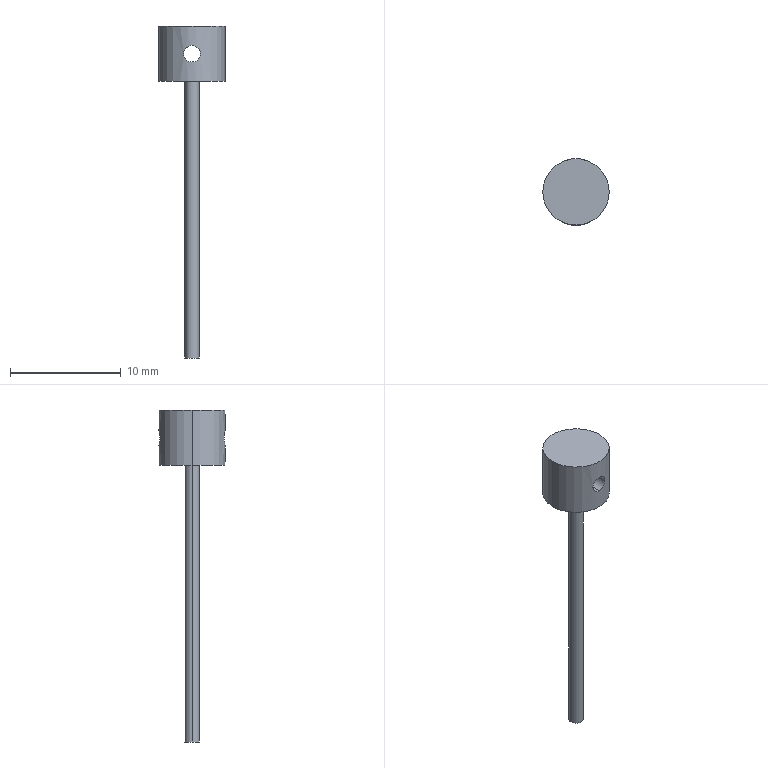Part | STEP file | detection pin | 1 solid | 9 faces | box 6 x 6 x 30 mm | volume 164.036 mm3 | cylinder 6 | plane 3 | commonest cylinder face diameters 1.3 x2 1.5 x2 6 x2
STEP:
#1=CARTESIAN_POINT('',(0.,0.,0.));
#2=DIRECTION('',(0.,0.,1.));
#3=DIRECTION('',(1.,0.,0.));
#4=AXIS2_PLACEMENT_3D('',#1,#2,#3);
#5=CARTESIAN_POINT('',(0.,3.,26.75));
#6=VERTEX_POINT('',#5);
#7=CARTESIAN_POINT('',(0.,-3.,26.75));
#8=VERTEX_POINT('',#7);
#9=CARTESIAN_POINT('',(0.,5.,26.75));
#10=DIRECTION('',(0.,-1.,0.));
#11=VECTOR('',#10,1.);
#12=LINE('',#9,#11);
#13=CARTESIAN_POINT('',(0.,5.,27.5));
#14=DIRECTION('',(0.,-1.,0.));
#15=DIRECTION('',(0.,0.,-1.));
#16=AXIS2_PLACEMENT_3D('',#13,#14,#15);
#17=CYLINDRICAL_SURFACE('',#16,0.75);
#18=CARTESIAN_POINT('',(6.283,0.));
#19=DIRECTION('',(0.,1.));
#20=VECTOR('',#19,1.);
#21=LINE('',#18,#20);
#22=(GEOMETRIC_REPRESENTATION_CONTEXT(2)PARAMETRIC_REPRESENTATION_CONTEXT()REPRESENTATION_CONTEXT('',''));
#23=DEFINITIONAL_REPRESENTATION('',(#21),#22);
#24=PCURVE('',#17,#23);
#25=CARTESIAN_POINT('',(0.,5.,27.5));
#26=DIRECTION('',(0.,-1.,0.));
#27=DIRECTION('',(0.,0.,-1.));
#28=AXIS2_PLACEMENT_3D('',#25,#26,#27);
#29=CYLINDRICAL_SURFACE('',#28,0.75);
#30=CARTESIAN_POINT('',(0.,0.));
#31=DIRECTION('',(0.,1.));
#32=VECTOR('',#31,1.);
#33=LINE('',#30,#32);
#34=(GEOMETRIC_REPRESENTATION_CONTEXT(2)PARAMETRIC_REPRESENTATION_CONTEXT()REPRESENTATION_CONTEXT('',''));
#35=DEFINITIONAL_REPRESENTATION('',(#33),#34);
#36=PCURVE('',#29,#35);
#37=SURFACE_CURVE('',#12,(#24,#36),.PCURVE_S1.);
#38=EDGE_CURVE('',#6,#8,#37,.T.);
#39=ORIENTED_EDGE('',*,*,#38,.T.);
#40=CARTESIAN_POINT('',(0.,-3.,28.25));
#41=VERTEX_POINT('',#40);
#42=CARTESIAN_POINT('',(0.,-3.,28.25));
#43=CARTESIAN_POINT('',(-0.0981,-3.,28.25));
#44=CARTESIAN_POINT('',(-0.1972,-2.995,28.23));
#45=CARTESIAN_POINT('',(-0.3778,-2.977,28.155));
#46=CARTESIAN_POINT('',(-0.4609,-2.965,28.1));
#47=CARTESIAN_POINT('',(-0.6685,-2.928,27.892));
#48=CARTESIAN_POINT('',(-0.7499,-2.905,27.698));
#49=CARTESIAN_POINT('',(-0.7501,-2.905,27.302));
#50=CARTESIAN_POINT('',(-0.6682,-2.928,27.108));
#51=CARTESIAN_POINT('',(-0.3931,-2.977,26.832));
#52=CARTESIAN_POINT('',(-0.199,-3.,26.75));
#53=CARTESIAN_POINT('',(0.,-3.,26.75));
#54=B_SPLINE_CURVE_WITH_KNOTS('',3,(#42,#43,#44,#45,#46,#47,#48,#49,#50,#51,#52,#53),.UNSPECIFIED.,.F.,.F.,(4,2,2,2,2,4),(0.002354,0.002648,0.002943,0.003531,0.004119,0.004708),.UNSPECIFIED.);
#55=CARTESIAN_POINT('',(3.142,8.));
#56=CARTESIAN_POINT('',(3.189,8.));
#57=CARTESIAN_POINT('',(3.285,7.999));
#58=CARTESIAN_POINT('',(3.428,7.993));
#59=CARTESIAN_POINT('',(3.571,7.984));
#60=CARTESIAN_POINT('',(3.713,7.973));
#61=CARTESIAN_POINT('',(3.855,7.96));
#62=CARTESIAN_POINT('',(3.998,7.946));
#63=CARTESIAN_POINT('',(4.14,7.933));
#64=CARTESIAN_POINT('',(4.283,7.922));
#65=CARTESIAN_POINT('',(4.425,7.912));
#66=CARTESIAN_POINT('',(4.568,7.906));
#67=CARTESIAN_POINT('',(4.712,7.904));
#68=CARTESIAN_POINT('',(4.856,7.906));
#69=CARTESIAN_POINT('',(4.999,7.912));
#70=CARTESIAN_POINT('',(5.142,7.922));
#71=CARTESIAN_POINT('',(5.284,7.933));
#72=CARTESIAN_POINT('',(5.426,7.946));
#73=CARTESIAN_POINT('',(5.568,7.96));
#74=CARTESIAN_POINT('',(5.71,7.972));
#75=CARTESIAN_POINT('',(5.852,7.984));
#76=CARTESIAN_POINT('',(5.995,7.993));
#77=CARTESIAN_POINT('',(6.139,7.999));
#78=CARTESIAN_POINT('',(6.235,8.));
#79=CARTESIAN_POINT('',(6.283,8.));
#80=B_SPLINE_CURVE_WITH_KNOTS('',3,(#55,#56,#57,#58,#59,#60,#61,#62,#63,#64,#65,#66,#67,#68,#69,#70,#71,#72,#73,#74,#75,#76,#77,#78,#79),.UNSPECIFIED.,.F.,.F.,(4,1,1,1,1,1,1,1,1,1,1,1,1,1,1,1,1,1,1,1,1,1,4),(0.002354,0.002461,0.002568,0.002675,0.002782,0.002889,0.002996,0.003103,0.00321,0.003317,0.003424,0.003531,0.003638,0.003745,0.003852,0.003959,0.004066,0.004173,0.00428,0.004387,0.004494,0.004601,0.004708),.QUASI_UNIFORM_KNOTS.);
#81=(GEOMETRIC_REPRESENTATION_CONTEXT(2)PARAMETRIC_REPRESENTATION_CONTEXT()REPRESENTATION_CONTEXT('',''));
#82=DEFINITIONAL_REPRESENTATION('',(#80),#81);
#83=PCURVE('',#17,#82);
#84=CARTESIAN_POINT('',(0.,0.,30.));
#85=DIRECTION('',(0.,0.,-1.));
#86=DIRECTION('',(-1.,0.,0.));
#87=AXIS2_PLACEMENT_3D('',#84,#85,#86);
#88=CYLINDRICAL_SURFACE('',#87,3.);
#89=CARTESIAN_POINT('',(4.712,1.75));
#90=CARTESIAN_POINT('',(4.724,1.75));
#91=CARTESIAN_POINT('',(4.748,1.755));
#92=CARTESIAN_POINT('',(4.783,1.778));
#93=CARTESIAN_POINT('',(4.817,1.816));
#94=CARTESIAN_POINT('',(4.848,1.867));
#95=CARTESIAN_POINT('',(4.877,1.931));
#96=CARTESIAN_POINT('',(4.903,2.007));
#97=CARTESIAN_POINT('',(4.925,2.093));
#98=CARTESIAN_POINT('',(4.942,2.187));
#99=CARTESIAN_POINT('',(4.955,2.287));
#100=CARTESIAN_POINT('',(4.963,2.392));
#101=CARTESIAN_POINT('',(4.966,2.5));
#102=CARTESIAN_POINT('',(4.963,2.608));
#103=CARTESIAN_POINT('',(4.955,2.713));
#104=CARTESIAN_POINT('',(4.942,2.813));
#105=CARTESIAN_POINT('',(4.925,2.907));
#106=CARTESIAN_POINT('',(4.903,2.993));
#107=CARTESIAN_POINT('',(4.878,3.068));
#108=CARTESIAN_POINT('',(4.849,3.132));
#109=CARTESIAN_POINT('',(4.817,3.183));
#110=CARTESIAN_POINT('',(4.784,3.221));
#111=CARTESIAN_POINT('',(4.748,3.245));
#112=CARTESIAN_POINT('',(4.724,3.25));
#113=CARTESIAN_POINT('',(4.712,3.25));
#114=B_SPLINE_CURVE_WITH_KNOTS('',3,(#89,#90,#91,#92,#93,#94,#95,#96,#97,#98,#99,#100,#101,#102,#103,#104,#105,#106,#107,#108,#109,#110,#111,#112,#113),.UNSPECIFIED.,.F.,.F.,(4,1,1,1,1,1,1,1,1,1,1,1,1,1,1,1,1,1,1,1,1,1,4),(0.002354,0.002461,0.002568,0.002675,0.002782,0.002889,0.002996,0.003103,0.00321,0.003317,0.003424,0.003531,0.003638,0.003745,0.003852,0.003959,0.004066,0.004173,0.00428,0.004387,0.004494,0.004601,0.004708),.QUASI_UNIFORM_KNOTS.);
#115=(GEOMETRIC_REPRESENTATION_CONTEXT(2)PARAMETRIC_REPRESENTATION_CONTEXT()REPRESENTATION_CONTEXT('',''));
#116=DEFINITIONAL_REPRESENTATION('',(#114),#115);
#117=PCURVE('',#88,#116);
#118=SURFACE_CURVE('',#54,(#83,#117),.PCURVE_S1.);
#119=EDGE_CURVE('',#41,#8,#118,.T.);
#120=ORIENTED_EDGE('',*,*,#119,.F.);
#121=CARTESIAN_POINT('',(0.,3.,28.25));
#122=VERTEX_POINT('',#121);
#123=CARTESIAN_POINT('',(0.,5.,28.25));
#124=DIRECTION('',(0.,-1.,0.));
#125=VECTOR('',#124,1.);
#126=LINE('',#123,#125);
#127=CARTESIAN_POINT('',(3.142,0.));
#128=DIRECTION('',(0.,1.));
#129=VECTOR('',#128,1.);
#130=LINE('',#127,#129);
#131=(GEOMETRIC_REPRESENTATION_CONTEXT(2)PARAMETRIC_REPRESENTATION_CONTEXT()REPRESENTATION_CONTEXT('',''));
#132=DEFINITIONAL_REPRESENTATION('',(#130),#131);
#133=PCURVE('',#17,#132);
#134=CARTESIAN_POINT('',(3.142,0.));
#135=DIRECTION('',(0.,1.));
#136=VECTOR('',#135,1.);
#137=LINE('',#134,#136);
#138=(GEOMETRIC_REPRESENTATION_CONTEXT(2)PARAMETRIC_REPRESENTATION_CONTEXT()REPRESENTATION_CONTEXT('',''));
#139=DEFINITIONAL_REPRESENTATION('',(#137),#138);
#140=PCURVE('',#29,#139);
#141=SURFACE_CURVE('',#126,(#133,#140),.PCURVE_S1.);
#142=EDGE_CURVE('',#122,#41,#141,.T.);
#143=ORIENTED_EDGE('',*,*,#142,.F.);
#144=CARTESIAN_POINT('',(0.,3.,26.75));
#145=CARTESIAN_POINT('',(-0.09953,3.,26.75));
#146=CARTESIAN_POINT('',(-0.1972,2.995,26.77));
#147=CARTESIAN_POINT('',(-0.3787,2.977,26.845));
#148=CARTESIAN_POINT('',(-0.4616,2.965,26.901));
#149=CARTESIAN_POINT('',(-0.5994,2.94,27.039));
#150=CARTESIAN_POINT('',(-0.6552,2.928,27.122));
#151=CARTESIAN_POINT('',(-0.7301,2.91,27.302));
#152=CARTESIAN_POINT('',(-0.75,2.905,27.401));
#153=CARTESIAN_POINT('',(-0.75,2.905,27.598));
#154=CARTESIAN_POINT('',(-0.7305,2.91,27.696));
#155=CARTESIAN_POINT('',(-0.6549,2.928,27.879));
#156=CARTESIAN_POINT('',(-0.5997,2.94,27.961));
#157=CARTESIAN_POINT('',(-0.4607,2.965,28.1));
#158=CARTESIAN_POINT('',(-0.3781,2.977,28.155));
#159=CARTESIAN_POINT('',(-0.197,2.995,28.23));
#160=CARTESIAN_POINT('',(-0.09813,3.,28.25));
#161=CARTESIAN_POINT('',(0.,3.,28.25));
#162=B_SPLINE_CURVE_WITH_KNOTS('',3,(#144,#145,#146,#147,#148,#149,#150,#151,#152,#153,#154,#155,#156,#157,#158,#159,#160,#161),.UNSPECIFIED.,.F.,.F.,(4,2,2,2,2,2,2,2,4),(0.,0.0002943,0.0005886,0.0008828,0.001177,0.001471,0.001766,0.00206,0.002354),.UNSPECIFIED.);
#163=CARTESIAN_POINT('',(6.283,2.));
#164=CARTESIAN_POINT('',(6.259,2.));
#165=CARTESIAN_POINT('',(6.211,2.));
#166=CARTESIAN_POINT('',(6.139,2.002));
#167=CARTESIAN_POINT('',(6.068,2.004));
#168=CARTESIAN_POINT('',(5.996,2.007));
#169=CARTESIAN_POINT('',(5.925,2.011));
#170=CARTESIAN_POINT('',(5.853,2.016));
#171=CARTESIAN_POINT('',(5.782,2.022));
#172=CARTESIAN_POINT('',(5.711,2.028));
#173=CARTESIAN_POINT('',(5.639,2.034));
#174=CARTESIAN_POINT('',(5.568,2.041));
#175=CARTESIAN_POINT('',(5.497,2.047));
#176=CARTESIAN_POINT('',(5.427,2.054));
#177=CARTESIAN_POINT('',(5.355,2.061));
#178=CARTESIAN_POINT('',(5.284,2.067));
#179=CARTESIAN_POINT('',(5.213,2.073));
#180=CARTESIAN_POINT('',(5.142,2.079));
#181=CARTESIAN_POINT('',(5.071,2.084));
#182=CARTESIAN_POINT('',(4.999,2.088));
#183=CARTESIAN_POINT('',(4.928,2.091));
#184=CARTESIAN_POINT('',(4.856,2.093));
#185=CARTESIAN_POINT('',(4.784,2.095));
#186=CARTESIAN_POINT('',(4.713,2.095));
#187=CARTESIAN_POINT('',(4.641,2.095));
#188=CARTESIAN_POINT('',(4.57,2.093));
#189=CARTESIAN_POINT('',(4.498,2.091));
#190=CARTESIAN_POINT('',(4.427,2.088));
#191=CARTESIAN_POINT('',(4.355,2.084));
#192=CARTESIAN_POINT('',(4.283,2.079));
#193=CARTESIAN_POINT('',(4.212,2.073));
#194=CARTESIAN_POINT('',(4.141,2.067));
#195=CARTESIAN_POINT('',(4.069,2.061));
#196=CARTESIAN_POINT('',(3.998,2.054));
#197=CARTESIAN_POINT('',(3.927,2.047));
#198=CARTESIAN_POINT('',(3.855,2.04));
#199=CARTESIAN_POINT('',(3.784,2.034));
#200=CARTESIAN_POINT('',(3.713,2.027));
#201=CARTESIAN_POINT('',(3.642,2.022));
#202=CARTESIAN_POINT('',(3.571,2.016));
#203=CARTESIAN_POINT('',(3.499,2.011));
#204=CARTESIAN_POINT('',(3.428,2.007));
#205=CARTESIAN_POINT('',(3.356,2.004));
#206=CARTESIAN_POINT('',(3.285,2.002));
#207=CARTESIAN_POINT('',(3.213,2.));
#208=CARTESIAN_POINT('',(3.165,2.));
#209=CARTESIAN_POINT('',(3.142,2.));
#210=B_SPLINE_CURVE_WITH_KNOTS('',3,(#163,#164,#165,#166,#167,#168,#169,#170,#171,#172,#173,#174,#175,#176,#177,#178,#179,#180,#181,#182,#183,#184,#185,#186,#187,#188,#189,#190,#191,#192,#193,#194,#195,#196,#197,#198,#199,#200,#201,#202,#203,#204,#205,#206,#207,#208,#209),.UNSPECIFIED.,.F.,.F.,(4,1,1,1,1,1,1,1,1,1,1,1,1,1,1,1,1,1,1,1,1,1,1,1,1,1,1,1,1,1,1,1,1,1,1,1,1,1,1,1,1,1,1,1,4),(0.,0.0000535,0.000107,0.0001605,0.000214,0.0002675,0.000321,0.0003745,0.000428,0.0004815,0.000535,0.0005886,0.0006421,0.0006956,0.0007491,0.0008026,0.0008561,0.0009096,0.0009631,0.001017,0.00107,0.001124,0.001177,0.001231,0.001284,0.001338,0.001391,0.001445,0.001498,0.001552,0.001605,0.001659,0.001712,0.001766,0.001819,0.001873,0.001926,0.00198,0.002033,0.002087,0.00214,0.002194,0.002247,0.002301,0.002354),.QUASI_UNIFORM_KNOTS.);
#211=(GEOMETRIC_REPRESENTATION_CONTEXT(2)PARAMETRIC_REPRESENTATION_CONTEXT()REPRESENTATION_CONTEXT('',''));
#212=DEFINITIONAL_REPRESENTATION('',(#210),#211);
#213=PCURVE('',#17,#212);
#214=CARTESIAN_POINT('',(0.,0.,30.));
#215=DIRECTION('',(0.,0.,-1.));
#216=DIRECTION('',(-1.,0.,0.));
#217=AXIS2_PLACEMENT_3D('',#214,#215,#216);
#218=CYLINDRICAL_SURFACE('',#217,3.);
#219=CARTESIAN_POINT('',(1.571,3.25));
#220=CARTESIAN_POINT('',(1.565,3.25));
#221=CARTESIAN_POINT('',(1.553,3.249));
#222=CARTESIAN_POINT('',(1.535,3.243));
#223=CARTESIAN_POINT('',(1.517,3.233));
#224=CARTESIAN_POINT('',(1.5,3.22));
#225=CARTESIAN_POINT('',(1.483,3.203));
#226=CARTESIAN_POINT('',(1.466,3.182));
#227=CARTESIAN_POINT('',(1.45,3.158));
#228=CARTESIAN_POINT('',(1.435,3.131));
#229=CARTESIAN_POINT('',(1.42,3.1));
#230=CARTESIAN_POINT('',(1.406,3.067));
#231=CARTESIAN_POINT('',(1.393,3.031));
#232=CARTESIAN_POINT('',(1.381,2.992));
#233=CARTESIAN_POINT('',(1.369,2.95));
#234=CARTESIAN_POINT('',(1.359,2.906));
#235=CARTESIAN_POINT('',(1.349,2.86));
#236=CARTESIAN_POINT('',(1.341,2.812));
#237=CARTESIAN_POINT('',(1.334,2.763));
#238=CARTESIAN_POINT('',(1.328,2.712));
#239=CARTESIAN_POINT('',(1.324,2.66));
#240=CARTESIAN_POINT('',(1.321,2.607));
#241=CARTESIAN_POINT('',(1.319,2.554));
#242=CARTESIAN_POINT('',(1.318,2.5));
#243=CARTESIAN_POINT('',(1.319,2.447));
#244=CARTESIAN_POINT('',(1.321,2.393));
#245=CARTESIAN_POINT('',(1.324,2.34));
#246=CARTESIAN_POINT('',(1.328,2.288));
#247=CARTESIAN_POINT('',(1.334,2.237));
#248=CARTESIAN_POINT('',(1.341,2.188));
#249=CARTESIAN_POINT('',(1.349,2.14));
#250=CARTESIAN_POINT('',(1.359,2.094));
#251=CARTESIAN_POINT('',(1.369,2.05));
#252=CARTESIAN_POINT('',(1.381,2.008));
#253=CARTESIAN_POINT('',(1.393,1.969));
#254=CARTESIAN_POINT('',(1.406,1.933));
#255=CARTESIAN_POINT('',(1.42,1.899));
#256=CARTESIAN_POINT('',(1.435,1.869));
#257=CARTESIAN_POINT('',(1.451,1.841));
#258=CARTESIAN_POINT('',(1.467,1.817));
#259=CARTESIAN_POINT('',(1.483,1.797));
#260=CARTESIAN_POINT('',(1.5,1.78));
#261=CARTESIAN_POINT('',(1.517,1.767));
#262=CARTESIAN_POINT('',(1.535,1.757));
#263=CARTESIAN_POINT('',(1.553,1.751));
#264=CARTESIAN_POINT('',(1.565,1.75));
#265=CARTESIAN_POINT('',(1.571,1.75));
#266=B_SPLINE_CURVE_WITH_KNOTS('',3,(#219,#220,#221,#222,#223,#224,#225,#226,#227,#228,#229,#230,#231,#232,#233,#234,#235,#236,#237,#238,#239,#240,#241,#242,#243,#244,#245,#246,#247,#248,#249,#250,#251,#252,#253,#254,#255,#256,#257,#258,#259,#260,#261,#262,#263,#264,#265),.UNSPECIFIED.,.F.,.F.,(4,1,1,1,1,1,1,1,1,1,1,1,1,1,1,1,1,1,1,1,1,1,1,1,1,1,1,1,1,1,1,1,1,1,1,1,1,1,1,1,1,1,1,1,4),(0.,0.0000535,0.000107,0.0001605,0.000214,0.0002675,0.000321,0.0003745,0.000428,0.0004815,0.000535,0.0005886,0.0006421,0.0006956,0.0007491,0.0008026,0.0008561,0.0009096,0.0009631,0.001017,0.00107,0.001124,0.001177,0.001231,0.001284,0.001338,0.001391,0.001445,0.001498,0.001552,0.001605,0.001659,0.001712,0.001766,0.001819,0.001873,0.001926,0.00198,0.002033,0.002087,0.00214,0.002194,0.002247,0.002301,0.002354),.QUASI_UNIFORM_KNOTS.);
#267=(GEOMETRIC_REPRESENTATION_CONTEXT(2)PARAMETRIC_REPRESENTATION_CONTEXT()REPRESENTATION_CONTEXT('',''));
#268=DEFINITIONAL_REPRESENTATION('',(#266),#267);
#269=PCURVE('',#218,#268);
#270=SURFACE_CURVE('',#162,(#213,#269),.PCURVE_S1.);
#271=EDGE_CURVE('',#6,#122,#270,.T.);
#272=ORIENTED_EDGE('',*,*,#271,.F.);
#273=EDGE_LOOP('',(#39,#120,#143,#272));
#274=FACE_BOUND('',#273,.F.);
#275=ADVANCED_FACE('',(#274),#17,.F.);
#276=CARTESIAN_POINT('',(0.65,0.,25.));
#277=VERTEX_POINT('',#276);
#278=CARTESIAN_POINT('',(-0.65,0.,25.));
#279=VERTEX_POINT('',#278);
#280=CARTESIAN_POINT('',(0.,0.,25.));
#281=DIRECTION('',(0.,0.,1.));
#282=DIRECTION('',(1.,0.,0.));
#283=AXIS2_PLACEMENT_3D('',#280,#281,#282);
#284=CIRCLE('',#283,0.65);
#285=CARTESIAN_POINT('',(0.,0.,25.));
#286=DIRECTION('',(0.,0.,-1.));
#287=DIRECTION('',(-1.,0.,0.));
#288=AXIS2_PLACEMENT_3D('',#285,#286,#287);
#289=CYLINDRICAL_SURFACE('',#288,0.65);
#290=CARTESIAN_POINT('',(3.142,0.));
#291=DIRECTION('',(-1.,0.));
#292=VECTOR('',#291,1.);
#293=LINE('',#290,#292);
#294=(GEOMETRIC_REPRESENTATION_CONTEXT(2)PARAMETRIC_REPRESENTATION_CONTEXT()REPRESENTATION_CONTEXT('',''));
#295=DEFINITIONAL_REPRESENTATION('',(#293),#294);
#296=PCURVE('',#289,#295);
#297=CARTESIAN_POINT('',(0.,0.,25.));
#298=DIRECTION('',(0.,0.,1.));
#299=DIRECTION('',(1.,0.,0.));
#300=AXIS2_PLACEMENT_3D('',#297,#298,#299);
#301=PLANE('',#300);
#302=CARTESIAN_POINT('',(0.,0.));
#303=DIRECTION('',(1.,0.));
#304=AXIS2_PLACEMENT_2D('',#302,#303);
#305=CIRCLE('',#304,0.65);
#306=(GEOMETRIC_REPRESENTATION_CONTEXT(2)PARAMETRIC_REPRESENTATION_CONTEXT()REPRESENTATION_CONTEXT('',''));
#307=DEFINITIONAL_REPRESENTATION('',(#305),#306);
#308=PCURVE('',#301,#307);
#309=SURFACE_CURVE('',#284,(#296,#308),.PCURVE_S1.);
#310=EDGE_CURVE('',#277,#279,#309,.T.);
#311=ORIENTED_EDGE('',*,*,#310,.F.);
#312=CARTESIAN_POINT('',(0.65,0.,0.));
#313=VERTEX_POINT('',#312);
#314=CARTESIAN_POINT('',(0.65,0.,25.));
#315=DIRECTION('',(0.,0.,-1.));
#316=VECTOR('',#315,1.);
#317=LINE('',#314,#316);
#318=CARTESIAN_POINT('',(3.142,0.));
#319=DIRECTION('',(0.,1.));
#320=VECTOR('',#319,1.);
#321=LINE('',#318,#320);
#322=(GEOMETRIC_REPRESENTATION_CONTEXT(2)PARAMETRIC_REPRESENTATION_CONTEXT()REPRESENTATION_CONTEXT('',''));
#323=DEFINITIONAL_REPRESENTATION('',(#321),#322);
#324=PCURVE('',#289,#323);
#325=CARTESIAN_POINT('',(0.,0.,25.));
#326=DIRECTION('',(0.,0.,-1.));
#327=DIRECTION('',(-1.,0.,0.));
#328=AXIS2_PLACEMENT_3D('',#325,#326,#327);
#329=CYLINDRICAL_SURFACE('',#328,0.65);
#330=CARTESIAN_POINT('',(3.142,0.));
#331=DIRECTION('',(0.,1.));
#332=VECTOR('',#331,1.);
#333=LINE('',#330,#332);
#334=(GEOMETRIC_REPRESENTATION_CONTEXT(2)PARAMETRIC_REPRESENTATION_CONTEXT()REPRESENTATION_CONTEXT('',''));
#335=DEFINITIONAL_REPRESENTATION('',(#333),#334);
#336=PCURVE('',#329,#335);
#337=SURFACE_CURVE('',#317,(#324,#336),.PCURVE_S1.);
#338=EDGE_CURVE('',#277,#313,#337,.T.);
#339=ORIENTED_EDGE('',*,*,#338,.T.);
#340=CARTESIAN_POINT('',(-0.65,0.,0.));
#341=VERTEX_POINT('',#340);
#342=CARTESIAN_POINT('',(0.,0.,0.));
#343=DIRECTION('',(0.,0.,1.));
#344=DIRECTION('',(1.,0.,0.));
#345=AXIS2_PLACEMENT_3D('',#342,#343,#344);
#346=CIRCLE('',#345,0.65);
#347=CARTESIAN_POINT('',(3.142,25.));
#348=DIRECTION('',(-1.,0.));
#349=VECTOR('',#348,1.);
#350=LINE('',#347,#349);
#351=(GEOMETRIC_REPRESENTATION_CONTEXT(2)PARAMETRIC_REPRESENTATION_CONTEXT()REPRESENTATION_CONTEXT('',''));
#352=DEFINITIONAL_REPRESENTATION('',(#350),#351);
#353=PCURVE('',#289,#352);
#354=CARTESIAN_POINT('',(0.,0.,0.));
#355=DIRECTION('',(0.,0.,1.));
#356=DIRECTION('',(1.,0.,0.));
#357=AXIS2_PLACEMENT_3D('',#354,#355,#356);
#358=PLANE('',#357);
#359=CARTESIAN_POINT('',(0.,0.));
#360=DIRECTION('',(1.,0.));
#361=AXIS2_PLACEMENT_2D('',#359,#360);
#362=CIRCLE('',#361,0.65);
#363=(GEOMETRIC_REPRESENTATION_CONTEXT(2)PARAMETRIC_REPRESENTATION_CONTEXT()REPRESENTATION_CONTEXT('',''));
#364=DEFINITIONAL_REPRESENTATION('',(#362),#363);
#365=PCURVE('',#358,#364);
#366=SURFACE_CURVE('',#346,(#353,#365),.PCURVE_S1.);
#367=EDGE_CURVE('',#313,#341,#366,.T.);
#368=ORIENTED_EDGE('',*,*,#367,.T.);
#369=CARTESIAN_POINT('',(-0.65,0.,25.));
#370=DIRECTION('',(0.,0.,-1.));
#371=VECTOR('',#370,1.);
#372=LINE('',#369,#371);
#373=CARTESIAN_POINT('',(0.,0.));
#374=DIRECTION('',(0.,1.));
#375=VECTOR('',#374,1.);
#376=LINE('',#373,#375);
#377=(GEOMETRIC_REPRESENTATION_CONTEXT(2)PARAMETRIC_REPRESENTATION_CONTEXT()REPRESENTATION_CONTEXT('',''));
#378=DEFINITIONAL_REPRESENTATION('',(#376),#377);
#379=PCURVE('',#289,#378);
#380=CARTESIAN_POINT('',(6.283,0.));
#381=DIRECTION('',(0.,1.));
#382=VECTOR('',#381,1.);
#383=LINE('',#380,#382);
#384=(GEOMETRIC_REPRESENTATION_CONTEXT(2)PARAMETRIC_REPRESENTATION_CONTEXT()REPRESENTATION_CONTEXT('',''));
#385=DEFINITIONAL_REPRESENTATION('',(#383),#384);
#386=PCURVE('',#329,#385);
#387=SURFACE_CURVE('',#372,(#379,#386),.PCURVE_S1.);
#388=EDGE_CURVE('',#279,#341,#387,.T.);
#389=ORIENTED_EDGE('',*,*,#388,.F.);
#390=EDGE_LOOP('',(#311,#339,#368,#389));
#391=FACE_BOUND('',#390,.T.);
#392=ADVANCED_FACE('',(#391),#289,.T.);
#393=ORIENTED_EDGE('',*,*,#271,.F.);
#394=CARTESIAN_POINT('',(0.,3.,28.25));
#395=CARTESIAN_POINT('',(0.0981,3.,28.25));
#396=CARTESIAN_POINT('',(0.1972,2.995,28.23));
#397=CARTESIAN_POINT('',(0.3778,2.977,28.155));
#398=CARTESIAN_POINT('',(0.4609,2.965,28.1));
#399=CARTESIAN_POINT('',(0.6685,2.928,27.892));
#400=CARTESIAN_POINT('',(0.7499,2.905,27.698));
#401=CARTESIAN_POINT('',(0.7501,2.905,27.302));
#402=CARTESIAN_POINT('',(0.6682,2.928,27.108));
#403=CARTESIAN_POINT('',(0.3931,2.977,26.832));
#404=CARTESIAN_POINT('',(0.199,3.,26.75));
#405=CARTESIAN_POINT('',(0.,3.,26.75));
#406=B_SPLINE_CURVE_WITH_KNOTS('',3,(#394,#395,#396,#397,#398,#399,#400,#401,#402,#403,#404,#405),.UNSPECIFIED.,.F.,.F.,(4,2,2,2,2,4),(0.002354,0.002648,0.002943,0.003531,0.004119,0.004708),.UNSPECIFIED.);
#407=CARTESIAN_POINT('',(1.571,1.75));
#408=CARTESIAN_POINT('',(1.583,1.75));
#409=CARTESIAN_POINT('',(1.607,1.755));
#410=CARTESIAN_POINT('',(1.642,1.778));
#411=CARTESIAN_POINT('',(1.675,1.816));
#412=CARTESIAN_POINT('',(1.707,1.867));
#413=CARTESIAN_POINT('',(1.736,1.931));
#414=CARTESIAN_POINT('',(1.761,2.007));
#415=CARTESIAN_POINT('',(1.783,2.093));
#416=CARTESIAN_POINT('',(1.801,2.187));
#417=CARTESIAN_POINT('',(1.814,2.287));
#418=CARTESIAN_POINT('',(1.822,2.392));
#419=CARTESIAN_POINT('',(1.824,2.5));
#420=CARTESIAN_POINT('',(1.822,2.608));
#421=CARTESIAN_POINT('',(1.814,2.713));
#422=CARTESIAN_POINT('',(1.801,2.813));
#423=CARTESIAN_POINT('',(1.783,2.907));
#424=CARTESIAN_POINT('',(1.761,2.993));
#425=CARTESIAN_POINT('',(1.736,3.068));
#426=CARTESIAN_POINT('',(1.707,3.132));
#427=CARTESIAN_POINT('',(1.676,3.183));
#428=CARTESIAN_POINT('',(1.642,3.221));
#429=CARTESIAN_POINT('',(1.607,3.245));
#430=CARTESIAN_POINT('',(1.583,3.25));
#431=CARTESIAN_POINT('',(1.571,3.25));
#432=B_SPLINE_CURVE_WITH_KNOTS('',3,(#407,#408,#409,#410,#411,#412,#413,#414,#415,#416,#417,#418,#419,#420,#421,#422,#423,#424,#425,#426,#427,#428,#429,#430,#431),.UNSPECIFIED.,.F.,.F.,(4,1,1,1,1,1,1,1,1,1,1,1,1,1,1,1,1,1,1,1,1,1,4),(0.002354,0.002461,0.002568,0.002675,0.002782,0.002889,0.002996,0.003103,0.00321,0.003317,0.003424,0.003531,0.003638,0.003745,0.003852,0.003959,0.004066,0.004173,0.00428,0.004387,0.004494,0.004601,0.004708),.QUASI_UNIFORM_KNOTS.);
#433=(GEOMETRIC_REPRESENTATION_CONTEXT(2)PARAMETRIC_REPRESENTATION_CONTEXT()REPRESENTATION_CONTEXT('',''));
#434=DEFINITIONAL_REPRESENTATION('',(#432),#433);
#435=PCURVE('',#218,#434);
#436=CARTESIAN_POINT('',(3.142,2.));
#437=CARTESIAN_POINT('',(3.094,2.));
#438=CARTESIAN_POINT('',(2.999,2.001));
#439=CARTESIAN_POINT('',(2.855,2.007));
#440=CARTESIAN_POINT('',(2.713,2.016));
#441=CARTESIAN_POINT('',(2.57,2.027));
#442=CARTESIAN_POINT('',(2.428,2.04));
#443=CARTESIAN_POINT('',(2.285,2.054));
#444=CARTESIAN_POINT('',(2.143,2.067));
#445=CARTESIAN_POINT('',(2.001,2.078));
#446=CARTESIAN_POINT('',(1.858,2.088));
#447=CARTESIAN_POINT('',(1.715,2.094));
#448=CARTESIAN_POINT('',(1.571,2.096));
#449=CARTESIAN_POINT('',(1.427,2.094));
#450=CARTESIAN_POINT('',(1.284,2.088));
#451=CARTESIAN_POINT('',(1.141,2.078));
#452=CARTESIAN_POINT('',(0.9987,2.067));
#453=CARTESIAN_POINT('',(0.8567,2.054));
#454=CARTESIAN_POINT('',(0.7152,2.04));
#455=CARTESIAN_POINT('',(0.5733,2.028));
#456=CARTESIAN_POINT('',(0.4308,2.016));
#457=CARTESIAN_POINT('',(0.2878,2.007));
#458=CARTESIAN_POINT('',(0.1443,2.001));
#459=CARTESIAN_POINT('',(0.04821,2.));
#460=CARTESIAN_POINT('',(0.,2.));
#461=B_SPLINE_CURVE_WITH_KNOTS('',3,(#436,#437,#438,#439,#440,#441,#442,#443,#444,#445,#446,#447,#448,#449,#450,#451,#452,#453,#454,#455,#456,#457,#458,#459,#460),.UNSPECIFIED.,.F.,.F.,(4,1,1,1,1,1,1,1,1,1,1,1,1,1,1,1,1,1,1,1,1,1,4),(0.002354,0.002461,0.002568,0.002675,0.002782,0.002889,0.002996,0.003103,0.00321,0.003317,0.003424,0.003531,0.003638,0.003745,0.003852,0.003959,0.004066,0.004173,0.00428,0.004387,0.004494,0.004601,0.004708),.QUASI_UNIFORM_KNOTS.);
#462=(GEOMETRIC_REPRESENTATION_CONTEXT(2)PARAMETRIC_REPRESENTATION_CONTEXT()REPRESENTATION_CONTEXT('',''));
#463=DEFINITIONAL_REPRESENTATION('',(#461),#462);
#464=PCURVE('',#29,#463);
#465=SURFACE_CURVE('',#406,(#435,#464),.PCURVE_S1.);
#466=EDGE_CURVE('',#122,#6,#465,.T.);
#467=ORIENTED_EDGE('',*,*,#466,.F.);
#468=EDGE_LOOP('',(#393,#467));
#469=FACE_BOUND('',#468,.T.);
#470=CARTESIAN_POINT('',(3.,0.,30.));
#471=VERTEX_POINT('',#470);
#472=CARTESIAN_POINT('',(-3.,0.,30.));
#473=VERTEX_POINT('',#472);
#474=CARTESIAN_POINT('',(0.,0.,30.));
#475=DIRECTION('',(0.,0.,1.));
#476=DIRECTION('',(1.,0.,0.));
#477=AXIS2_PLACEMENT_3D('',#474,#475,#476);
#478=CIRCLE('',#477,3.);
#479=CARTESIAN_POINT('',(3.142,0.));
#480=DIRECTION('',(-1.,0.));
#481=VECTOR('',#480,1.);
#482=LINE('',#479,#481);
#483=(GEOMETRIC_REPRESENTATION_CONTEXT(2)PARAMETRIC_REPRESENTATION_CONTEXT()REPRESENTATION_CONTEXT('',''));
#484=DEFINITIONAL_REPRESENTATION('',(#482),#483);
#485=PCURVE('',#218,#484);
#486=CARTESIAN_POINT('',(0.,0.,30.));
#487=DIRECTION('',(0.,0.,1.));
#488=DIRECTION('',(1.,0.,0.));
#489=AXIS2_PLACEMENT_3D('',#486,#487,#488);
#490=PLANE('',#489);
#491=CARTESIAN_POINT('',(0.,0.));
#492=DIRECTION('',(1.,0.));
#493=AXIS2_PLACEMENT_2D('',#491,#492);
#494=CIRCLE('',#493,3.);
#495=(GEOMETRIC_REPRESENTATION_CONTEXT(2)PARAMETRIC_REPRESENTATION_CONTEXT()REPRESENTATION_CONTEXT('',''));
#496=DEFINITIONAL_REPRESENTATION('',(#494),#495);
#497=PCURVE('',#490,#496);
#498=SURFACE_CURVE('',#478,(#485,#497),.PCURVE_S1.);
#499=EDGE_CURVE('',#471,#473,#498,.T.);
#500=ORIENTED_EDGE('',*,*,#499,.F.);
#501=CARTESIAN_POINT('',(3.,0.,25.));
#502=VERTEX_POINT('',#501);
#503=CARTESIAN_POINT('',(3.,0.,30.));
#504=DIRECTION('',(0.,0.,-1.));
#505=VECTOR('',#504,1.);
#506=LINE('',#503,#505);
#507=CARTESIAN_POINT('',(3.142,0.));
#508=DIRECTION('',(0.,1.));
#509=VECTOR('',#508,1.);
#510=LINE('',#507,#509);
#511=(GEOMETRIC_REPRESENTATION_CONTEXT(2)PARAMETRIC_REPRESENTATION_CONTEXT()REPRESENTATION_CONTEXT('',''));
#512=DEFINITIONAL_REPRESENTATION('',(#510),#511);
#513=PCURVE('',#218,#512);
#514=CARTESIAN_POINT('',(3.142,0.));
#515=DIRECTION('',(0.,1.));
#516=VECTOR('',#515,1.);
#517=LINE('',#514,#516);
#518=(GEOMETRIC_REPRESENTATION_CONTEXT(2)PARAMETRIC_REPRESENTATION_CONTEXT()REPRESENTATION_CONTEXT('',''));
#519=DEFINITIONAL_REPRESENTATION('',(#517),#518);
#520=PCURVE('',#88,#519);
#521=SURFACE_CURVE('',#506,(#513,#520),.PCURVE_S1.);
#522=EDGE_CURVE('',#471,#502,#521,.T.);
#523=ORIENTED_EDGE('',*,*,#522,.T.);
#524=CARTESIAN_POINT('',(-3.,0.,25.));
#525=VERTEX_POINT('',#524);
#526=CARTESIAN_POINT('',(0.,0.,25.));
#527=DIRECTION('',(0.,0.,1.));
#528=DIRECTION('',(1.,0.,0.));
#529=AXIS2_PLACEMENT_3D('',#526,#527,#528);
#530=CIRCLE('',#529,3.);
#531=CARTESIAN_POINT('',(3.142,5.));
#532=DIRECTION('',(-1.,0.));
#533=VECTOR('',#532,1.);
#534=LINE('',#531,#533);
#535=(GEOMETRIC_REPRESENTATION_CONTEXT(2)PARAMETRIC_REPRESENTATION_CONTEXT()REPRESENTATION_CONTEXT('',''));
#536=DEFINITIONAL_REPRESENTATION('',(#534),#535);
#537=PCURVE('',#218,#536);
#538=CARTESIAN_POINT('',(0.,0.));
#539=DIRECTION('',(1.,0.));
#540=AXIS2_PLACEMENT_2D('',#538,#539);
#541=CIRCLE('',#540,3.);
#542=(GEOMETRIC_REPRESENTATION_CONTEXT(2)PARAMETRIC_REPRESENTATION_CONTEXT()REPRESENTATION_CONTEXT('',''));
#543=DEFINITIONAL_REPRESENTATION('',(#541),#542);
#544=PCURVE('',#301,#543);
#545=SURFACE_CURVE('',#530,(#537,#544),.PCURVE_S1.);
#546=EDGE_CURVE('',#502,#525,#545,.T.);
#547=ORIENTED_EDGE('',*,*,#546,.T.);
#548=CARTESIAN_POINT('',(-3.,0.,30.));
#549=DIRECTION('',(0.,0.,-1.));
#550=VECTOR('',#549,1.);
#551=LINE('',#548,#550);
#552=CARTESIAN_POINT('',(0.,0.));
#553=DIRECTION('',(0.,1.));
#554=VECTOR('',#553,1.);
#555=LINE('',#552,#554);
#556=(GEOMETRIC_REPRESENTATION_CONTEXT(2)PARAMETRIC_REPRESENTATION_CONTEXT()REPRESENTATION_CONTEXT('',''));
#557=DEFINITIONAL_REPRESENTATION('',(#555),#556);
#558=PCURVE('',#218,#557);
#559=CARTESIAN_POINT('',(6.283,0.));
#560=DIRECTION('',(0.,1.));
#561=VECTOR('',#560,1.);
#562=LINE('',#559,#561);
#563=(GEOMETRIC_REPRESENTATION_CONTEXT(2)PARAMETRIC_REPRESENTATION_CONTEXT()REPRESENTATION_CONTEXT('',''));
#564=DEFINITIONAL_REPRESENTATION('',(#562),#563);
#565=PCURVE('',#88,#564);
#566=SURFACE_CURVE('',#551,(#558,#565),.PCURVE_S1.);
#567=EDGE_CURVE('',#473,#525,#566,.T.);
#568=ORIENTED_EDGE('',*,*,#567,.F.);
#569=EDGE_LOOP('',(#500,#523,#547,#568));
#570=FACE_BOUND('',#569,.T.);
#571=ADVANCED_FACE('',(#469,#570),#218,.T.);
#572=ORIENTED_EDGE('',*,*,#522,.F.);
#573=CARTESIAN_POINT('',(0.,0.,30.));
#574=DIRECTION('',(0.,0.,1.));
#575=DIRECTION('',(1.,0.,0.));
#576=AXIS2_PLACEMENT_3D('',#573,#574,#575);
#577=CIRCLE('',#576,3.);
#578=CARTESIAN_POINT('',(9.425,0.));
#579=DIRECTION('',(-1.,0.));
#580=VECTOR('',#579,1.);
#581=LINE('',#578,#580);
#582=(GEOMETRIC_REPRESENTATION_CONTEXT(2)PARAMETRIC_REPRESENTATION_CONTEXT()REPRESENTATION_CONTEXT('',''));
#583=DEFINITIONAL_REPRESENTATION('',(#581),#582);
#584=PCURVE('',#88,#583);
#585=CARTESIAN_POINT('',(0.,0.));
#586=DIRECTION('',(1.,0.));
#587=AXIS2_PLACEMENT_2D('',#585,#586);
#588=CIRCLE('',#587,3.);
#589=(GEOMETRIC_REPRESENTATION_CONTEXT(2)PARAMETRIC_REPRESENTATION_CONTEXT()REPRESENTATION_CONTEXT('',''));
#590=DEFINITIONAL_REPRESENTATION('',(#588),#589);
#591=PCURVE('',#490,#590);
#592=SURFACE_CURVE('',#577,(#584,#591),.PCURVE_S1.);
#593=EDGE_CURVE('',#473,#471,#592,.T.);
#594=ORIENTED_EDGE('',*,*,#593,.F.);
#595=ORIENTED_EDGE('',*,*,#567,.T.);
#596=CARTESIAN_POINT('',(0.,0.,25.));
#597=DIRECTION('',(0.,0.,1.));
#598=DIRECTION('',(1.,0.,0.));
#599=AXIS2_PLACEMENT_3D('',#596,#597,#598);
#600=CIRCLE('',#599,3.);
#601=CARTESIAN_POINT('',(9.425,5.));
#602=DIRECTION('',(-1.,0.));
#603=VECTOR('',#602,1.);
#604=LINE('',#601,#603);
#605=(GEOMETRIC_REPRESENTATION_CONTEXT(2)PARAMETRIC_REPRESENTATION_CONTEXT()REPRESENTATION_CONTEXT('',''));
#606=DEFINITIONAL_REPRESENTATION('',(#604),#605);
#607=PCURVE('',#88,#606);
#608=CARTESIAN_POINT('',(0.,0.));
#609=DIRECTION('',(1.,0.));
#610=AXIS2_PLACEMENT_2D('',#608,#609);
#611=CIRCLE('',#610,3.);
#612=(GEOMETRIC_REPRESENTATION_CONTEXT(2)PARAMETRIC_REPRESENTATION_CONTEXT()REPRESENTATION_CONTEXT('',''));
#613=DEFINITIONAL_REPRESENTATION('',(#611),#612);
#614=PCURVE('',#301,#613);
#615=SURFACE_CURVE('',#600,(#607,#614),.PCURVE_S1.);
#616=EDGE_CURVE('',#525,#502,#615,.T.);
#617=ORIENTED_EDGE('',*,*,#616,.T.);
#618=EDGE_LOOP('',(#572,#594,#595,#617));
#619=FACE_BOUND('',#618,.T.);
#620=CARTESIAN_POINT('',(0.,-3.,26.75));
#621=CARTESIAN_POINT('',(0.09953,-3.,26.75));
#622=CARTESIAN_POINT('',(0.1972,-2.995,26.77));
#623=CARTESIAN_POINT('',(0.3787,-2.977,26.845));
#624=CARTESIAN_POINT('',(0.4616,-2.965,26.901));
#625=CARTESIAN_POINT('',(0.5994,-2.94,27.039));
#626=CARTESIAN_POINT('',(0.6552,-2.928,27.122));
#627=CARTESIAN_POINT('',(0.7301,-2.91,27.302));
#628=CARTESIAN_POINT('',(0.75,-2.905,27.401));
#629=CARTESIAN_POINT('',(0.75,-2.905,27.598));
#630=CARTESIAN_POINT('',(0.7305,-2.91,27.696));
#631=CARTESIAN_POINT('',(0.6549,-2.928,27.879));
#632=CARTESIAN_POINT('',(0.5997,-2.94,27.961));
#633=CARTESIAN_POINT('',(0.4607,-2.965,28.1));
#634=CARTESIAN_POINT('',(0.3781,-2.977,28.155));
#635=CARTESIAN_POINT('',(0.197,-2.995,28.23));
#636=CARTESIAN_POINT('',(0.09813,-3.,28.25));
#637=CARTESIAN_POINT('',(0.,-3.,28.25));
#638=B_SPLINE_CURVE_WITH_KNOTS('',3,(#620,#621,#622,#623,#624,#625,#626,#627,#628,#629,#630,#631,#632,#633,#634,#635,#636,#637),.UNSPECIFIED.,.F.,.F.,(4,2,2,2,2,2,2,2,4),(0.,0.0002943,0.0005886,0.0008828,0.001177,0.001471,0.001766,0.00206,0.002354),.UNSPECIFIED.);
#639=CARTESIAN_POINT('',(4.712,3.25));
#640=CARTESIAN_POINT('',(4.706,3.25));
#641=CARTESIAN_POINT('',(4.694,3.249));
#642=CARTESIAN_POINT('',(4.676,3.243));
#643=CARTESIAN_POINT('',(4.659,3.233));
#644=CARTESIAN_POINT('',(4.642,3.22));
#645=CARTESIAN_POINT('',(4.625,3.203));
#646=CARTESIAN_POINT('',(4.608,3.182));
#647=CARTESIAN_POINT('',(4.592,3.158));
#648=CARTESIAN_POINT('',(4.576,3.131));
#649=CARTESIAN_POINT('',(4.562,3.1));
#650=CARTESIAN_POINT('',(4.548,3.067));
#651=CARTESIAN_POINT('',(4.534,3.031));
#652=CARTESIAN_POINT('',(4.522,2.992));
#653=CARTESIAN_POINT('',(4.511,2.95));
#654=CARTESIAN_POINT('',(4.5,2.906));
#655=CARTESIAN_POINT('',(4.491,2.86));
#656=CARTESIAN_POINT('',(4.483,2.812));
#657=CARTESIAN_POINT('',(4.476,2.763));
#658=CARTESIAN_POINT('',(4.47,2.712));
#659=CARTESIAN_POINT('',(4.465,2.66));
#660=CARTESIAN_POINT('',(4.462,2.607));
#661=CARTESIAN_POINT('',(4.46,2.554));
#662=CARTESIAN_POINT('',(4.459,2.5));
#663=CARTESIAN_POINT('',(4.46,2.447));
#664=CARTESIAN_POINT('',(4.462,2.393));
#665=CARTESIAN_POINT('',(4.465,2.34));
#666=CARTESIAN_POINT('',(4.47,2.288));
#667=CARTESIAN_POINT('',(4.476,2.237));
#668=CARTESIAN_POINT('',(4.483,2.188));
#669=CARTESIAN_POINT('',(4.491,2.14));
#670=CARTESIAN_POINT('',(4.5,2.094));
#671=CARTESIAN_POINT('',(4.511,2.05));
#672=CARTESIAN_POINT('',(4.522,2.008));
#673=CARTESIAN_POINT('',(4.535,1.969));
#674=CARTESIAN_POINT('',(4.548,1.933));
#675=CARTESIAN_POINT('',(4.562,1.899));
#676=CARTESIAN_POINT('',(4.577,1.869));
#677=CARTESIAN_POINT('',(4.592,1.841));
#678=CARTESIAN_POINT('',(4.608,1.817));
#679=CARTESIAN_POINT('',(4.625,1.797));
#680=CARTESIAN_POINT('',(4.642,1.78));
#681=CARTESIAN_POINT('',(4.659,1.767));
#682=CARTESIAN_POINT('',(4.677,1.757));
#683=CARTESIAN_POINT('',(4.695,1.751));
#684=CARTESIAN_POINT('',(4.706,1.75));
#685=CARTESIAN_POINT('',(4.712,1.75));
#686=B_SPLINE_CURVE_WITH_KNOTS('',3,(#639,#640,#641,#642,#643,#644,#645,#646,#647,#648,#649,#650,#651,#652,#653,#654,#655,#656,#657,#658,#659,#660,#661,#662,#663,#664,#665,#666,#667,#668,#669,#670,#671,#672,#673,#674,#675,#676,#677,#678,#679,#680,#681,#682,#683,#684,#685),.UNSPECIFIED.,.F.,.F.,(4,1,1,1,1,1,1,1,1,1,1,1,1,1,1,1,1,1,1,1,1,1,1,1,1,1,1,1,1,1,1,1,1,1,1,1,1,1,1,1,1,1,1,1,4),(0.,0.0000535,0.000107,0.0001605,0.000214,0.0002675,0.000321,0.0003745,0.000428,0.0004815,0.000535,0.0005886,0.0006421,0.0006956,0.0007491,0.0008026,0.0008561,0.0009096,0.0009631,0.001017,0.00107,0.001124,0.001177,0.001231,0.001284,0.001338,0.001391,0.001445,0.001498,0.001552,0.001605,0.001659,0.001712,0.001766,0.001819,0.001873,0.001926,0.00198,0.002033,0.002087,0.00214,0.002194,0.002247,0.002301,0.002354),.QUASI_UNIFORM_KNOTS.);
#687=(GEOMETRIC_REPRESENTATION_CONTEXT(2)PARAMETRIC_REPRESENTATION_CONTEXT()REPRESENTATION_CONTEXT('',''));
#688=DEFINITIONAL_REPRESENTATION('',(#686),#687);
#689=PCURVE('',#88,#688);
#690=CARTESIAN_POINT('',(0.,8.));
#691=CARTESIAN_POINT('',(0.02413,8.));
#692=CARTESIAN_POINT('',(0.07222,8.));
#693=CARTESIAN_POINT('',(0.144,7.998));
#694=CARTESIAN_POINT('',(0.2155,7.996));
#695=CARTESIAN_POINT('',(0.2869,7.993));
#696=CARTESIAN_POINT('',(0.3583,7.989));
#697=CARTESIAN_POINT('',(0.4298,7.984));
#698=CARTESIAN_POINT('',(0.5012,7.978));
#699=CARTESIAN_POINT('',(0.5725,7.972));
#700=CARTESIAN_POINT('',(0.6437,7.966));
#701=CARTESIAN_POINT('',(0.7148,7.959));
#702=CARTESIAN_POINT('',(0.7857,7.953));
#703=CARTESIAN_POINT('',(0.8566,7.946));
#704=CARTESIAN_POINT('',(0.9278,7.939));
#705=CARTESIAN_POINT('',(0.9991,7.933));
#706=CARTESIAN_POINT('',(1.07,7.927));
#707=CARTESIAN_POINT('',(1.142,7.921));
#708=CARTESIAN_POINT('',(1.213,7.916));
#709=CARTESIAN_POINT('',(1.284,7.912));
#710=CARTESIAN_POINT('',(1.355,7.909));
#711=CARTESIAN_POINT('',(1.427,7.907));
#712=CARTESIAN_POINT('',(1.499,7.905));
#713=CARTESIAN_POINT('',(1.57,7.905));
#714=CARTESIAN_POINT('',(1.642,7.905));
#715=CARTESIAN_POINT('',(1.713,7.907));
#716=CARTESIAN_POINT('',(1.785,7.909));
#717=CARTESIAN_POINT('',(1.857,7.912));
#718=CARTESIAN_POINT('',(1.928,7.916));
#719=CARTESIAN_POINT('',(2.,7.921));
#720=CARTESIAN_POINT('',(2.071,7.927));
#721=CARTESIAN_POINT('',(2.143,7.933));
#722=CARTESIAN_POINT('',(2.214,7.939));
#723=CARTESIAN_POINT('',(2.285,7.946));
#724=CARTESIAN_POINT('',(2.356,7.953));
#725=CARTESIAN_POINT('',(2.428,7.96));
#726=CARTESIAN_POINT('',(2.499,7.966));
#727=CARTESIAN_POINT('',(2.57,7.973));
#728=CARTESIAN_POINT('',(2.641,7.978));
#729=CARTESIAN_POINT('',(2.713,7.984));
#730=CARTESIAN_POINT('',(2.784,7.989));
#731=CARTESIAN_POINT('',(2.855,7.993));
#732=CARTESIAN_POINT('',(2.927,7.996));
#733=CARTESIAN_POINT('',(2.999,7.998));
#734=CARTESIAN_POINT('',(3.07,8.));
#735=CARTESIAN_POINT('',(3.118,8.));
#736=CARTESIAN_POINT('',(3.142,8.));
#737=B_SPLINE_CURVE_WITH_KNOTS('',3,(#690,#691,#692,#693,#694,#695,#696,#697,#698,#699,#700,#701,#702,#703,#704,#705,#706,#707,#708,#709,#710,#711,#712,#713,#714,#715,#716,#717,#718,#719,#720,#721,#722,#723,#724,#725,#726,#727,#728,#729,#730,#731,#732,#733,#734,#735,#736),.UNSPECIFIED.,.F.,.F.,(4,1,1,1,1,1,1,1,1,1,1,1,1,1,1,1,1,1,1,1,1,1,1,1,1,1,1,1,1,1,1,1,1,1,1,1,1,1,1,1,1,1,1,1,4),(0.,0.0000535,0.000107,0.0001605,0.000214,0.0002675,0.000321,0.0003745,0.000428,0.0004815,0.000535,0.0005886,0.0006421,0.0006956,0.0007491,0.0008026,0.0008561,0.0009096,0.0009631,0.001017,0.00107,0.001124,0.001177,0.001231,0.001284,0.001338,0.001391,0.001445,0.001498,0.001552,0.001605,0.001659,0.001712,0.001766,0.001819,0.001873,0.001926,0.00198,0.002033,0.002087,0.00214,0.002194,0.002247,0.002301,0.002354),.QUASI_UNIFORM_KNOTS.);
#738=(GEOMETRIC_REPRESENTATION_CONTEXT(2)PARAMETRIC_REPRESENTATION_CONTEXT()REPRESENTATION_CONTEXT('',''));
#739=DEFINITIONAL_REPRESENTATION('',(#737),#738);
#740=PCURVE('',#29,#739);
#741=SURFACE_CURVE('',#638,(#689,#740),.PCURVE_S1.);
#742=EDGE_CURVE('',#8,#41,#741,.T.);
#743=ORIENTED_EDGE('',*,*,#742,.F.);
#744=ORIENTED_EDGE('',*,*,#119,.F.);
#745=EDGE_LOOP('',(#743,#744));
#746=FACE_BOUND('',#745,.T.);
#747=ADVANCED_FACE('',(#619,#746),#88,.T.);
#748=ORIENTED_EDGE('',*,*,#338,.F.);
#749=CARTESIAN_POINT('',(0.,0.,25.));
#750=DIRECTION('',(0.,0.,1.));
#751=DIRECTION('',(1.,0.,0.));
#752=AXIS2_PLACEMENT_3D('',#749,#750,#751);
#753=CIRCLE('',#752,0.65);
#754=CARTESIAN_POINT('',(9.425,0.));
#755=DIRECTION('',(-1.,0.));
#756=VECTOR('',#755,1.);
#757=LINE('',#754,#756);
#758=(GEOMETRIC_REPRESENTATION_CONTEXT(2)PARAMETRIC_REPRESENTATION_CONTEXT()REPRESENTATION_CONTEXT('',''));
#759=DEFINITIONAL_REPRESENTATION('',(#757),#758);
#760=PCURVE('',#329,#759);
#761=CARTESIAN_POINT('',(0.,0.));
#762=DIRECTION('',(1.,0.));
#763=AXIS2_PLACEMENT_2D('',#761,#762);
#764=CIRCLE('',#763,0.65);
#765=(GEOMETRIC_REPRESENTATION_CONTEXT(2)PARAMETRIC_REPRESENTATION_CONTEXT()REPRESENTATION_CONTEXT('',''));
#766=DEFINITIONAL_REPRESENTATION('',(#764),#765);
#767=PCURVE('',#301,#766);
#768=SURFACE_CURVE('',#753,(#760,#767),.PCURVE_S1.);
#769=EDGE_CURVE('',#279,#277,#768,.T.);
#770=ORIENTED_EDGE('',*,*,#769,.F.);
#771=ORIENTED_EDGE('',*,*,#388,.T.);
#772=CARTESIAN_POINT('',(0.,0.,0.));
#773=DIRECTION('',(0.,0.,1.));
#774=DIRECTION('',(1.,0.,0.));
#775=AXIS2_PLACEMENT_3D('',#772,#773,#774);
#776=CIRCLE('',#775,0.65);
#777=CARTESIAN_POINT('',(9.425,25.));
#778=DIRECTION('',(-1.,0.));
#779=VECTOR('',#778,1.);
#780=LINE('',#777,#779);
#781=(GEOMETRIC_REPRESENTATION_CONTEXT(2)PARAMETRIC_REPRESENTATION_CONTEXT()REPRESENTATION_CONTEXT('',''));
#782=DEFINITIONAL_REPRESENTATION('',(#780),#781);
#783=PCURVE('',#329,#782);
#784=CARTESIAN_POINT('',(0.,0.));
#785=DIRECTION('',(1.,0.));
#786=AXIS2_PLACEMENT_2D('',#784,#785);
#787=CIRCLE('',#786,0.65);
#788=(GEOMETRIC_REPRESENTATION_CONTEXT(2)PARAMETRIC_REPRESENTATION_CONTEXT()REPRESENTATION_CONTEXT('',''));
#789=DEFINITIONAL_REPRESENTATION('',(#787),#788);
#790=PCURVE('',#358,#789);
#791=SURFACE_CURVE('',#776,(#783,#790),.PCURVE_S1.);
#792=EDGE_CURVE('',#341,#313,#791,.T.);
#793=ORIENTED_EDGE('',*,*,#792,.T.);
#794=EDGE_LOOP('',(#748,#770,#771,#793));
#795=FACE_BOUND('',#794,.T.);
#796=ADVANCED_FACE('',(#795),#329,.T.);
#797=ORIENTED_EDGE('',*,*,#792,.F.);
#798=ORIENTED_EDGE('',*,*,#367,.F.);
#799=EDGE_LOOP('',(#797,#798));
#800=FACE_BOUND('',#799,.T.);
#801=ADVANCED_FACE('',(#800),#358,.F.);
#802=ORIENTED_EDGE('',*,*,#616,.F.);
#803=ORIENTED_EDGE('',*,*,#546,.F.);
#804=EDGE_LOOP('',(#802,#803));
#805=FACE_BOUND('',#804,.T.);
#806=ORIENTED_EDGE('',*,*,#769,.T.);
#807=ORIENTED_EDGE('',*,*,#310,.T.);
#808=EDGE_LOOP('',(#806,#807));
#809=FACE_BOUND('',#808,.T.);
#810=ADVANCED_FACE('',(#805,#809),#301,.F.);
#811=ORIENTED_EDGE('',*,*,#593,.T.);
#812=ORIENTED_EDGE('',*,*,#499,.T.);
#813=EDGE_LOOP('',(#811,#812));
#814=FACE_BOUND('',#813,.T.);
#815=ADVANCED_FACE('',(#814),#490,.T.);
#816=ORIENTED_EDGE('',*,*,#742,.F.);
#817=ORIENTED_EDGE('',*,*,#38,.F.);
#818=ORIENTED_EDGE('',*,*,#466,.F.);
#819=ORIENTED_EDGE('',*,*,#142,.T.);
#820=EDGE_LOOP('',(#816,#817,#818,#819));
#821=FACE_BOUND('',#820,.F.);
#822=ADVANCED_FACE('',(#821),#29,.F.);
#823=CLOSED_SHELL('',(#275,#392,#571,#747,#796,#801,#810,#815,#822));
#824=MANIFOLD_SOLID_BREP('',#823);
#825=(LENGTH_UNIT()NAMED_UNIT(*)SI_UNIT(.MILLI.,.METRE.));
#826=UNCERTAINTY_MEASURE_WITH_UNIT(LENGTH_MEASURE(0.0002),#825,'','');
#827=(NAMED_UNIT(*)PLANE_ANGLE_UNIT()SI_UNIT($,.RADIAN.));
#828=(NAMED_UNIT(*)SI_UNIT($,.STERADIAN.)SOLID_ANGLE_UNIT());
#829=(GEOMETRIC_REPRESENTATION_CONTEXT(3)GLOBAL_UNCERTAINTY_ASSIGNED_CONTEXT((#826))GLOBAL_UNIT_ASSIGNED_CONTEXT((#825,#827,#828))REPRESENTATION_CONTEXT('',''));
#830=ADVANCED_BREP_SHAPE_REPRESENTATION('',(#4,#824),#829);